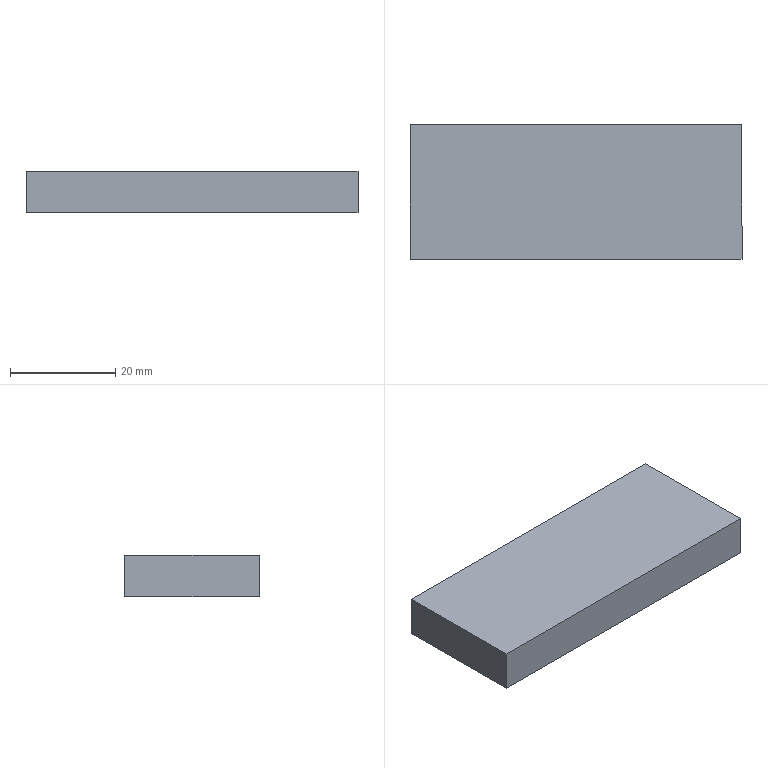Part | STEP file | 垫块5- | 1 solid | 6 faces | box 63 x 25.5 x 7.95 mm | volume 12772 mm3 | plane 6
STEP:
#1=CARTESIAN_POINT('',(63.,0.,7.95));
#2=VERTEX_POINT('',#1);
#3=CARTESIAN_POINT('',(63.,25.5,7.95));
#4=VERTEX_POINT('',#3);
#5=CARTESIAN_POINT('',(63.,25.5,7.95));
#6=DIRECTION('',(0.,1.,0.));
#7=VECTOR('',#6,1000.);
#8=LINE('',#5,#7);
#9=EDGE_CURVE('',#2,#4,#8,.T.);
#10=ORIENTED_EDGE('',*,*,#9,.F.);
#11=CARTESIAN_POINT('',(63.,0.,0.));
#12=VERTEX_POINT('',#11);
#13=CARTESIAN_POINT('',(63.,0.,75.915));
#14=DIRECTION('',(0.,0.,-1.));
#15=VECTOR('',#14,1000.);
#16=LINE('',#13,#15);
#17=EDGE_CURVE('',#2,#12,#16,.T.);
#18=ORIENTED_EDGE('',*,*,#17,.T.);
#19=CARTESIAN_POINT('',(63.,25.5,0.));
#20=VERTEX_POINT('',#19);
#21=CARTESIAN_POINT('',(63.,25.5,0.));
#22=DIRECTION('',(0.,1.,0.));
#23=VECTOR('',#22,1000.);
#24=LINE('',#21,#23);
#25=EDGE_CURVE('',#12,#20,#24,.T.);
#26=ORIENTED_EDGE('',*,*,#25,.T.);
#27=CARTESIAN_POINT('',(63.,25.5,75.915));
#28=DIRECTION('',(0.,0.,-1.));
#29=VECTOR('',#28,1000.);
#30=LINE('',#27,#29);
#31=EDGE_CURVE('',#4,#20,#30,.T.);
#32=ORIENTED_EDGE('',*,*,#31,.F.);
#33=EDGE_LOOP('',(#10,#18,#26,#32));
#34=FACE_OUTER_BOUND('',#33,.T.);
#35=CARTESIAN_POINT('',(63.,25.5,75.915));
#36=DIRECTION('',(-1.,0.,0.));
#37=DIRECTION('',(0.,-1.,0.));
#38=AXIS2_PLACEMENT_3D('',#35,#36,#37);
#39=PLANE('',#38);
#40=ADVANCED_FACE('',(#34),#39,.F.);
#41=CARTESIAN_POINT('',(0.,25.5,7.95));
#42=VERTEX_POINT('',#41);
#43=CARTESIAN_POINT('',(63.,25.5,7.95));
#44=DIRECTION('',(-1.,0.,0.));
#45=VECTOR('',#44,1000.);
#46=LINE('',#43,#45);
#47=EDGE_CURVE('',#4,#42,#46,.T.);
#48=ORIENTED_EDGE('',*,*,#47,.F.);
#49=ORIENTED_EDGE('',*,*,#31,.T.);
#50=CARTESIAN_POINT('',(0.,25.5,0.));
#51=VERTEX_POINT('',#50);
#52=CARTESIAN_POINT('',(63.,25.5,0.));
#53=DIRECTION('',(-1.,0.,0.));
#54=VECTOR('',#53,1000.);
#55=LINE('',#52,#54);
#56=EDGE_CURVE('',#20,#51,#55,.T.);
#57=ORIENTED_EDGE('',*,*,#56,.T.);
#58=CARTESIAN_POINT('',(0.,25.5,75.915));
#59=DIRECTION('',(0.,0.,-1.));
#60=VECTOR('',#59,1000.);
#61=LINE('',#58,#60);
#62=EDGE_CURVE('',#42,#51,#61,.T.);
#63=ORIENTED_EDGE('',*,*,#62,.F.);
#64=EDGE_LOOP('',(#48,#49,#57,#63));
#65=FACE_OUTER_BOUND('',#64,.T.);
#66=CARTESIAN_POINT('',(63.,25.5,75.915));
#67=DIRECTION('',(0.,-1.,0.));
#68=DIRECTION('',(0.,0.,-1.));
#69=AXIS2_PLACEMENT_3D('',#66,#67,#68);
#70=PLANE('',#69);
#71=ADVANCED_FACE('',(#65),#70,.F.);
#72=CARTESIAN_POINT('',(0.,0.,7.95));
#73=VERTEX_POINT('',#72);
#74=CARTESIAN_POINT('',(0.,25.5,7.95));
#75=DIRECTION('',(0.,-1.,0.));
#76=VECTOR('',#75,1000.);
#77=LINE('',#74,#76);
#78=EDGE_CURVE('',#42,#73,#77,.T.);
#79=ORIENTED_EDGE('',*,*,#78,.F.);
#80=ORIENTED_EDGE('',*,*,#62,.T.);
#81=CARTESIAN_POINT('',(0.,0.,0.));
#82=VERTEX_POINT('',#81);
#83=CARTESIAN_POINT('',(0.,25.5,0.));
#84=DIRECTION('',(0.,-1.,0.));
#85=VECTOR('',#84,1000.);
#86=LINE('',#83,#85);
#87=EDGE_CURVE('',#51,#82,#86,.T.);
#88=ORIENTED_EDGE('',*,*,#87,.T.);
#89=CARTESIAN_POINT('',(0.,0.,75.915));
#90=DIRECTION('',(0.,0.,-1.));
#91=VECTOR('',#90,1000.);
#92=LINE('',#89,#91);
#93=EDGE_CURVE('',#73,#82,#92,.T.);
#94=ORIENTED_EDGE('',*,*,#93,.F.);
#95=EDGE_LOOP('',(#79,#80,#88,#94));
#96=FACE_OUTER_BOUND('',#95,.T.);
#97=CARTESIAN_POINT('',(0.,25.5,75.915));
#98=DIRECTION('',(1.,0.,0.));
#99=DIRECTION('',(0.,1.,0.));
#100=AXIS2_PLACEMENT_3D('',#97,#98,#99);
#101=PLANE('',#100);
#102=ADVANCED_FACE('',(#96),#101,.F.);
#103=CARTESIAN_POINT('',(63.,0.,7.95));
#104=DIRECTION('',(1.,0.,0.));
#105=VECTOR('',#104,1000.);
#106=LINE('',#103,#105);
#107=EDGE_CURVE('',#73,#2,#106,.T.);
#108=ORIENTED_EDGE('',*,*,#107,.F.);
#109=ORIENTED_EDGE('',*,*,#93,.T.);
#110=CARTESIAN_POINT('',(63.,0.,0.));
#111=DIRECTION('',(1.,0.,0.));
#112=VECTOR('',#111,1000.);
#113=LINE('',#110,#112);
#114=EDGE_CURVE('',#82,#12,#113,.T.);
#115=ORIENTED_EDGE('',*,*,#114,.T.);
#116=ORIENTED_EDGE('',*,*,#17,.F.);
#117=EDGE_LOOP('',(#108,#109,#115,#116));
#118=FACE_OUTER_BOUND('',#117,.T.);
#119=CARTESIAN_POINT('',(63.,0.,75.915));
#120=DIRECTION('',(0.,1.,0.));
#121=DIRECTION('',(-1.,0.,0.));
#122=AXIS2_PLACEMENT_3D('',#119,#120,#121);
#123=PLANE('',#122);
#124=ADVANCED_FACE('',(#118),#123,.F.);
#125=ORIENTED_EDGE('',*,*,#25,.F.);
#126=ORIENTED_EDGE('',*,*,#114,.F.);
#127=ORIENTED_EDGE('',*,*,#87,.F.);
#128=ORIENTED_EDGE('',*,*,#56,.F.);
#129=EDGE_LOOP('',(#125,#126,#127,#128));
#130=FACE_OUTER_BOUND('',#129,.T.);
#131=CARTESIAN_POINT('',(0.,0.,0.));
#132=DIRECTION('',(0.,0.,-1.));
#133=DIRECTION('',(-1.,0.,0.));
#134=AXIS2_PLACEMENT_3D('',#131,#132,#133);
#135=PLANE('',#134);
#136=ADVANCED_FACE('',(#130),#135,.T.);
#137=ORIENTED_EDGE('',*,*,#107,.T.);
#138=ORIENTED_EDGE('',*,*,#9,.T.);
#139=ORIENTED_EDGE('',*,*,#47,.T.);
#140=ORIENTED_EDGE('',*,*,#78,.T.);
#141=EDGE_LOOP('',(#137,#138,#139,#140));
#142=FACE_OUTER_BOUND('',#141,.T.);
#143=CARTESIAN_POINT('',(-62.,7.25,7.95));
#144=DIRECTION('',(0.,0.,1.));
#145=DIRECTION('',(-1.,0.,0.));
#146=AXIS2_PLACEMENT_3D('',#143,#144,#145);
#147=PLANE('',#146);
#148=ADVANCED_FACE('',(#142),#147,.T.);
#149=CLOSED_SHELL('',(#40,#71,#102,#124,#136,#148));
#150=MANIFOLD_SOLID_BREP('',#149);
#151=CARTESIAN_POINT('',(0.,0.,0.));
#152=DIRECTION('',(0.,0.,1.));
#153=DIRECTION('',(1.,0.,0.));
#154=AXIS2_PLACEMENT_3D('',#151,#152,#153);
#155=(LENGTH_UNIT()NAMED_UNIT(*)SI_UNIT(.MILLI.,.METRE.));
#156=UNCERTAINTY_MEASURE_WITH_UNIT(LENGTH_MEASURE(0.00001),#155,'','');
#157=(NAMED_UNIT(*)PLANE_ANGLE_UNIT()SI_UNIT($,.RADIAN.));
#158=(NAMED_UNIT(*)SI_UNIT($,.STERADIAN.)SOLID_ANGLE_UNIT());
#159=(GEOMETRIC_REPRESENTATION_CONTEXT(3)GLOBAL_UNCERTAINTY_ASSIGNED_CONTEXT((#156))GLOBAL_UNIT_ASSIGNED_CONTEXT((#155,#157,#158))REPRESENTATION_CONTEXT('',''));
#160=ADVANCED_BREP_SHAPE_REPRESENTATION('',(#150,#154),#159);